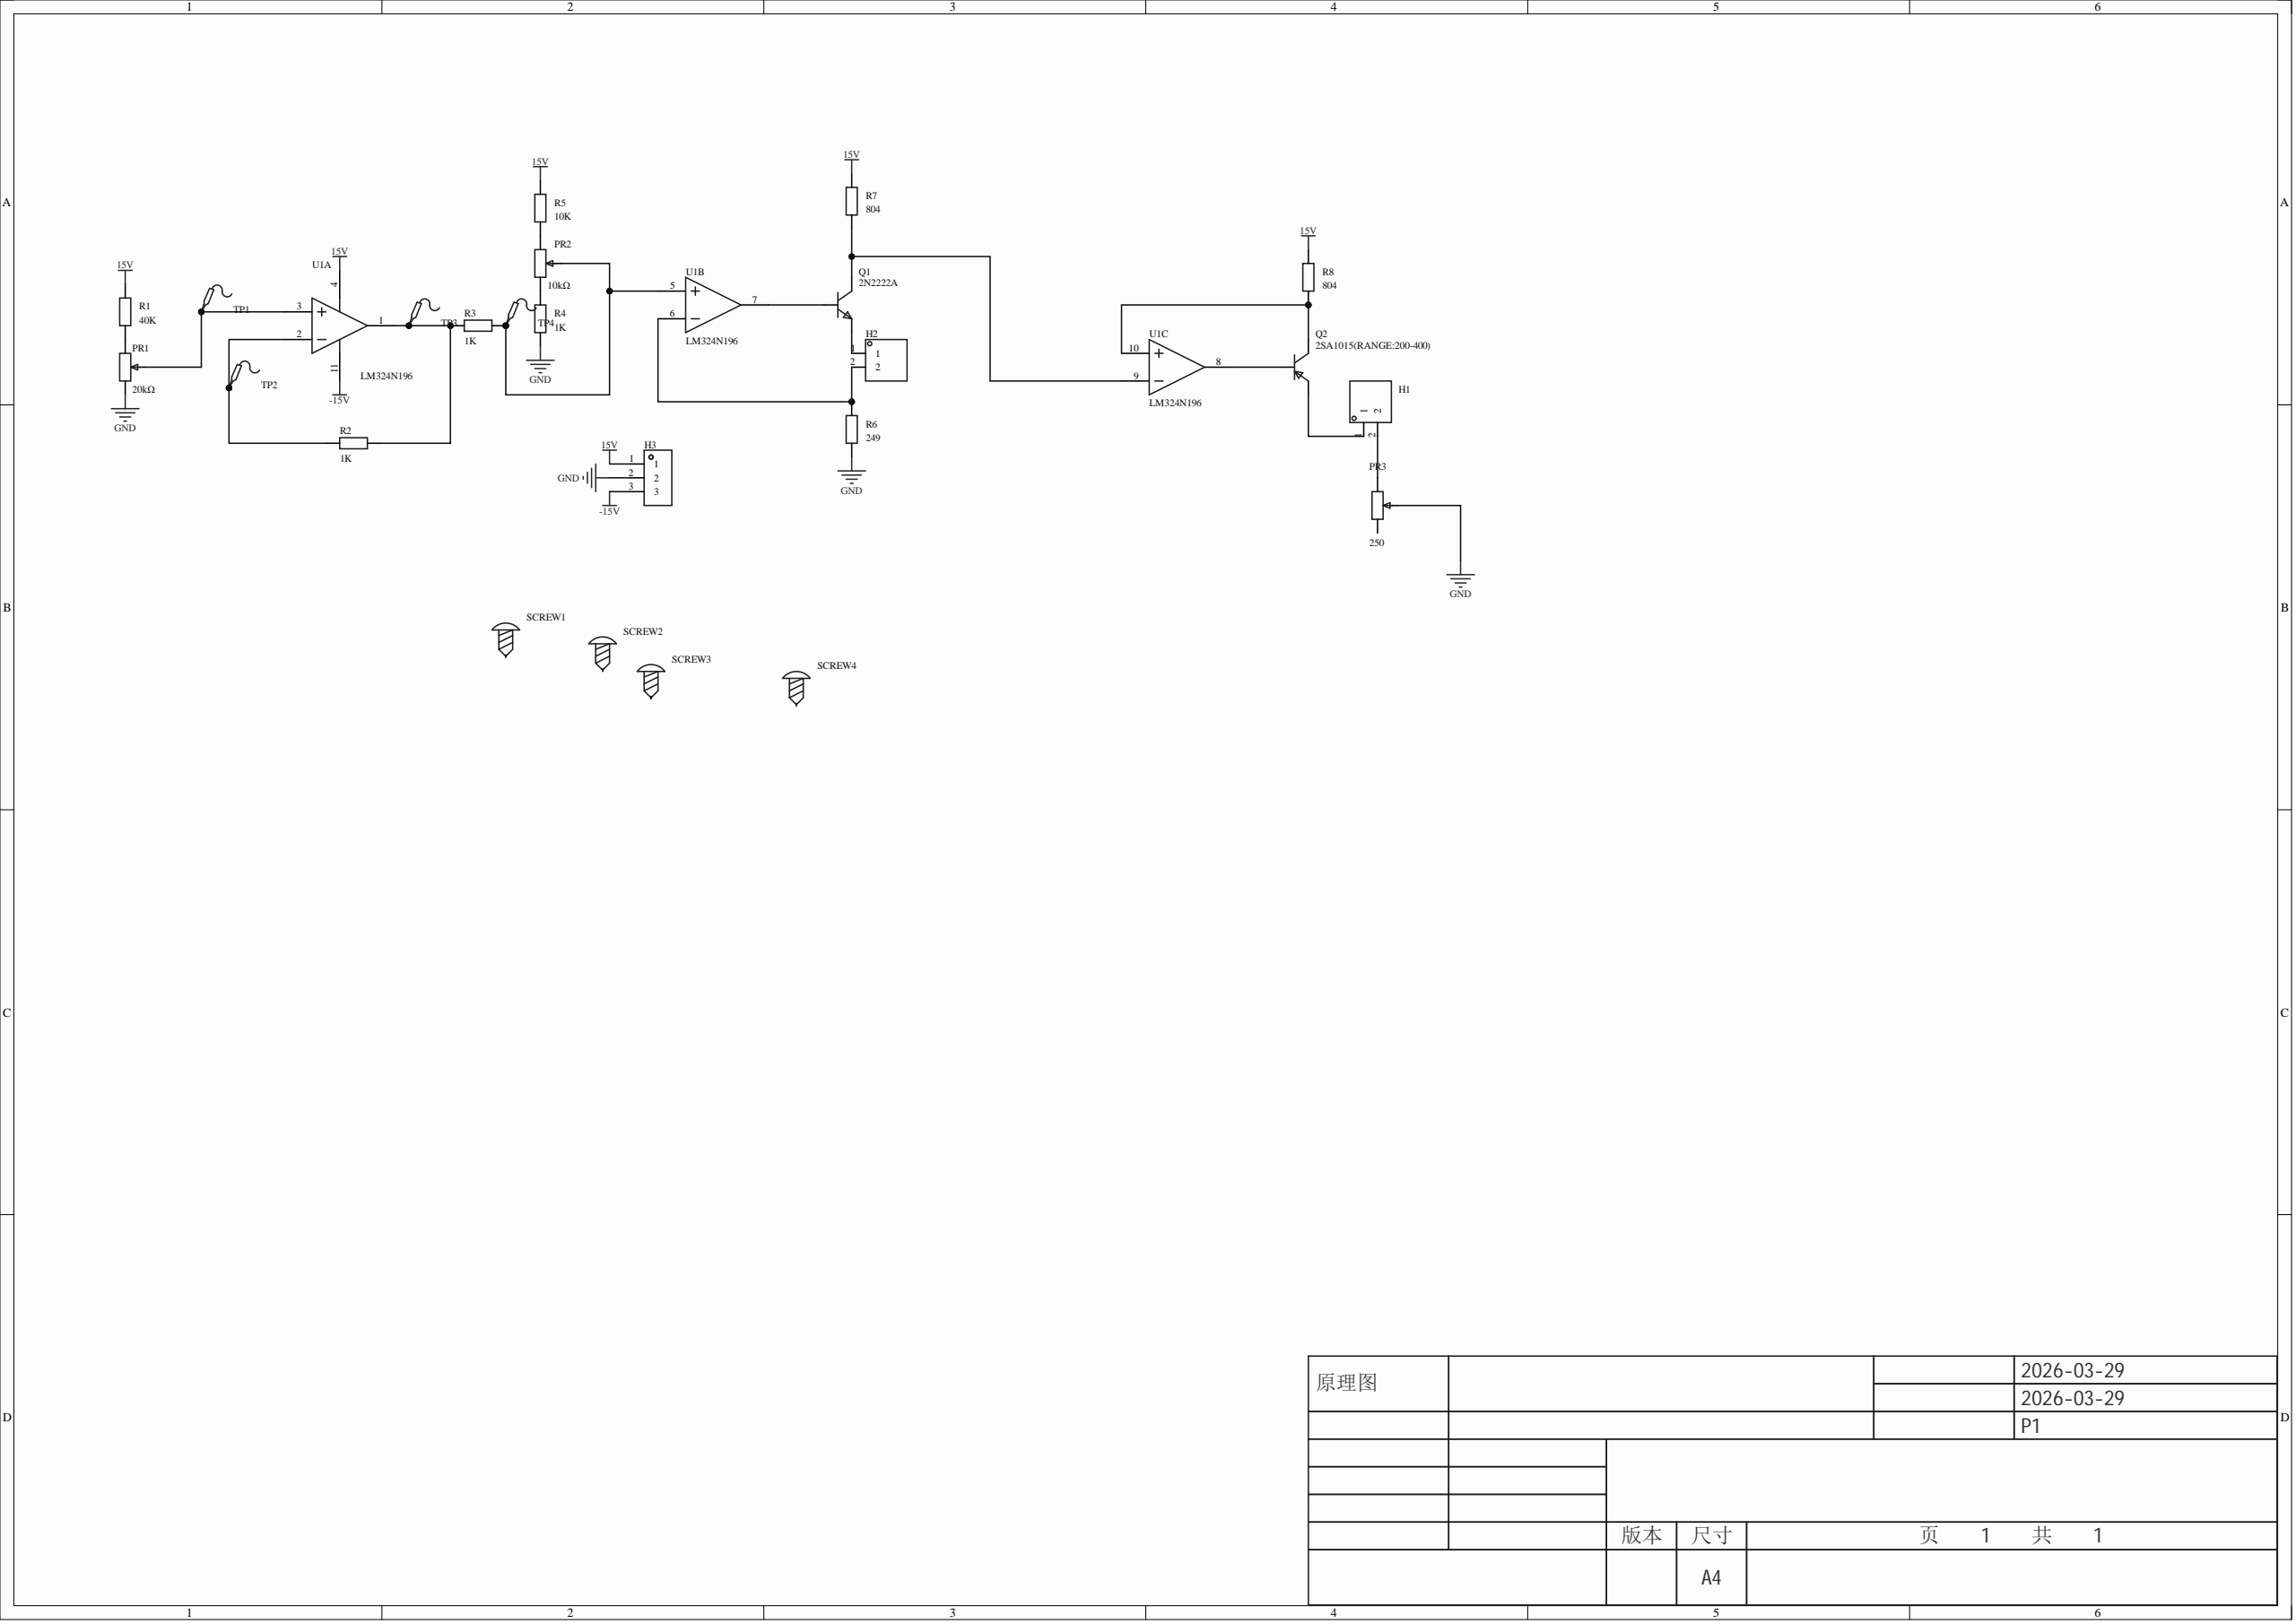Circuit board | Altium Designer | 25 parts | 18 nets
Bill of materials:
Comment,Description,Designator,Footprint,LibRef,Quantity
"","","H1, H2","HDR-TH_2P-P2.54-V-M-1","HDR-M_2.54_1x2P","2"
"","","H3","HDR-TH_3P-P2.54-V-M","HDR-M_2.54_1x3P","1"
"20kΩ","","PR1","R_3296","R_3296","1"
"10kΩ","","PR2","R_3296","R_3296","1"
"250","","PR3","R_3296","R_3296","1"
"2N2222A","","Q1","TO-92-3_L5.1-W4.1-P1.27-L-1","2N2222A_C50229645","1"
"2SA1015(RANGE:200-400)","","Q2","TO-92-3_L4.9-W3.7-P1.27-L","2SA1015(RANGE:200-400)","1"
"40K","","R1","R0805","Res_0805","1"
"1K","","R2, R3, R4","R0805","Res_0805","3"
"10K","","R5","R0805","Res_0805","1"
"249","","R6","R0805","Res_0805","1"
"804","","R7, R8","R0805","Res_0805","2"
"","","SCREW1, SCREW2, SCREW3, SCREW4","M2螺丝","M2螺丝","4"
"","","TP1, TP2, TP3, TP4","Test-Point-0.5mm","Test-Point","4"
"LM324N196","","U1","PDIP-14_L19.3-W6.5-P2.54-LS7.6-BL","LM324N196","1"
Netlist (Protel format):
[
H1
HDR-TH_2P-P2.54-V-M-1




]
[
H2
HDR-TH_2P-P2.54-V-M-1




]
[
H3
HDR-TH_3P-P2.54-V-M




]
[
PR1
R_3296
20kΩ



]
[
PR2
R_3296
10kΩ



]
[
PR3
R_3296
250



]
[
Q1
TO-92-3_L5.1-W4.1-P1.27-L-1
2N2222A



]
[
Q2
TO-92-3_L4.9-W3.7-P1.27-L
2SA1015(RANGE:200-400)



]
[
R1
R0805
40K



]
[
R2
R0805
1K



]
[
R3
R0805
1K



]
[
R4
R0805
1K



]
[
R5
R0805
10K



]
[
R6
R0805
249



]
[
R7
R0805
804



]
[
R8
R0805
804



]
[
SCREW1
M2螺丝




]
[
SCREW2
M2螺丝




]
[
SCREW3
M2螺丝




]
[
SCREW4
M2螺丝




]
[
TP1
Test-Point-0.5mm




]
[
TP2
Test-Point-0.5mm




]
[
TP3
Test-Point-0.5mm




]
[
TP4
Test-Point-0.5mm




]
[
U1
PDIP-14_L19.3-W6.5-P2.54-LS7.6-BL
LM324N196



]
(
NetR2_2
R2-2
TP2-1
U1-2
)
(
NetR2_1
R2-1
R3-2
TP3-1
U1-1
)
(
NetQ2_3
Q2-3
U1-8
)
(
NetQ2_2
Q2-2
R8-2
U1-10
)
(
NetQ1_3
Q1-3
R7-2
U1-9
)
(
NetQ1_2
Q1-2
U1-7
)
(
NetPR2_3
PR2-3
R5-2
)
(
NetPR2_2
PR2-2
R3-1
TP4-1
U1-5
)
(
NetPR2_1
PR2-1
R4-1
)
(
NetPR1_3
PR1-3
R1-1
)
(
NetPR1_2
PR1-2
TP1-1
U1-3
)
(
NetH2_2
H2-2
R6-1
U1-6
)
(
NetH2_1
H2-1
Q1-1
)
(
NetH1_2
H1-2
PR3-3
)
(
NetH1_1
H1-1
Q2-1
)
(
GND
H3-2
PR1-1
PR3-2
R4-2
R6-2
)
(
-15V
H3-3
U1-11
)
(
15V
H3-1
R1-2
R5-1
R7-1
R8-1
U1-4
)